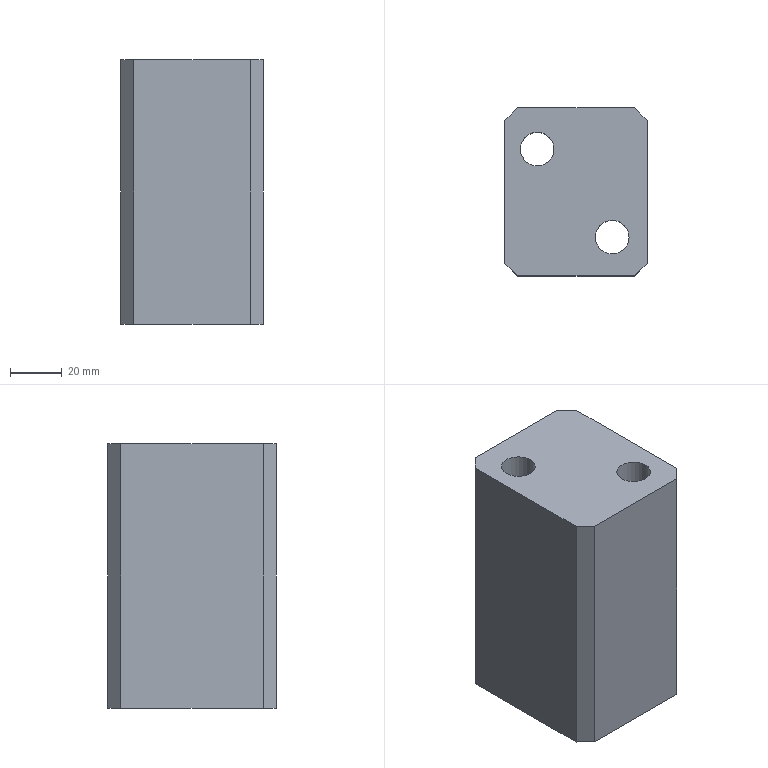Part | STEP file | gslz 2016.10.28-10_id2074_x_t | 1 solid | 22 faces | box 55 x 65 x 102 mm | volume 303943 mm3 | plane 12 | cylinder 6 | cone 4 | commonest cylinder face diameters 10.3 x2 13 x2 20 x2
STEP:
#1=CARTESIAN_POINT('',(0.,0.,0.));
#2=DIRECTION('',(0.,0.,1.));
#3=DIRECTION('',(1.,0.,0.));
#4=AXIS2_PLACEMENT_3D('',#1,#2,#3);
#5=CARTESIAN_POINT('',(512.5,-304.,3.));
#6=VERTEX_POINT('',#5);
#7=CARTESIAN_POINT('',(506.5,-304.,3.));
#8=DIRECTION('',(0.,0.,-1.));
#9=DIRECTION('',(1.,0.,0.));
#10=AXIS2_PLACEMENT_3D('',#7,#8,#9);
#11=CIRCLE('',#10,6.);
#12=CARTESIAN_POINT('',(501.5,-310.,3.));
#13=DIRECTION('',(0.,0.,1.));
#14=DIRECTION('',(0.,-1.,0.));
#15=AXIS2_PLACEMENT_3D('',#12,#13,#14);
#16=PLANE('',#15);
#17=CARTESIAN_POINT('',(-6.,11.));
#18=CARTESIAN_POINT('',(4.392,11.));
#19=CARTESIAN_POINT('',(-0.8038,2.));
#20=CARTESIAN_POINT('',(-6.,-7.));
#21=CARTESIAN_POINT('',(-11.196,2.));
#22=CARTESIAN_POINT('',(-16.392,11.));
#23=CARTESIAN_POINT('',(-6.,11.));
#24=(BOUNDED_CURVE()B_SPLINE_CURVE(2,(#17,#18,#19,#20,#21,#22,#23),.UNSPECIFIED.,.T.,.F.)B_SPLINE_CURVE_WITH_KNOTS((1,2,2,2,2,1),(-2.094,0.,2.094,4.189,6.283,8.378),.UNSPECIFIED.)CURVE()GEOMETRIC_REPRESENTATION_ITEM()RATIONAL_B_SPLINE_CURVE((1.,0.5,1.,0.5,1.,0.5,1.))REPRESENTATION_ITEM(''));
#25=(GEOMETRIC_REPRESENTATION_CONTEXT(2)PARAMETRIC_REPRESENTATION_CONTEXT()REPRESENTATION_CONTEXT('',''));
#26=DEFINITIONAL_REPRESENTATION('',(#24),#25);
#27=PCURVE('',#16,#26);
#28=CARTESIAN_POINT('',(506.5,-304.,3.));
#29=DIRECTION('',(0.,0.,-1.));
#30=DIRECTION('',(1.,0.,0.));
#31=AXIS2_PLACEMENT_3D('',#28,#29,#30);
#32=CONICAL_SURFACE('',#31,6.,0.7854);
#33=CARTESIAN_POINT('',(0.,0.));
#34=DIRECTION('',(1.,0.));
#35=VECTOR('',#34,1.);
#36=LINE('',#33,#35);
#37=(GEOMETRIC_REPRESENTATION_CONTEXT(2)PARAMETRIC_REPRESENTATION_CONTEXT()REPRESENTATION_CONTEXT('',''));
#38=DEFINITIONAL_REPRESENTATION('',(#36),#37);
#39=PCURVE('',#32,#38);
#40=SURFACE_CURVE('',#11,(#27,#39),.PCURVE_S1.);
#41=EDGE_CURVE('',#6,#6,#40,.T.);
#42=ORIENTED_EDGE('',*,*,#41,.F.);
#43=EDGE_LOOP('',(#42));
#44=FACE_BOUND('',#43,.T.);
#45=CARTESIAN_POINT('',(541.5,-269.,3.));
#46=VERTEX_POINT('',#45);
#47=CARTESIAN_POINT('',(535.5,-269.,3.));
#48=DIRECTION('',(0.,0.,-1.));
#49=DIRECTION('',(1.,0.,0.));
#50=AXIS2_PLACEMENT_3D('',#47,#48,#49);
#51=CIRCLE('',#50,6.);
#52=CARTESIAN_POINT('',(-41.,40.));
#53=CARTESIAN_POINT('',(-30.608,40.));
#54=CARTESIAN_POINT('',(-35.804,31.));
#55=CARTESIAN_POINT('',(-41.,22.));
#56=CARTESIAN_POINT('',(-46.196,31.));
#57=CARTESIAN_POINT('',(-51.392,40.));
#58=CARTESIAN_POINT('',(-41.,40.));
#59=(BOUNDED_CURVE()B_SPLINE_CURVE(2,(#52,#53,#54,#55,#56,#57,#58),.UNSPECIFIED.,.T.,.F.)B_SPLINE_CURVE_WITH_KNOTS((1,2,2,2,2,1),(-2.094,0.,2.094,4.189,6.283,8.378),.UNSPECIFIED.)CURVE()GEOMETRIC_REPRESENTATION_ITEM()RATIONAL_B_SPLINE_CURVE((1.,0.5,1.,0.5,1.,0.5,1.))REPRESENTATION_ITEM(''));
#60=(GEOMETRIC_REPRESENTATION_CONTEXT(2)PARAMETRIC_REPRESENTATION_CONTEXT()REPRESENTATION_CONTEXT('',''));
#61=DEFINITIONAL_REPRESENTATION('',(#59),#60);
#62=PCURVE('',#16,#61);
#63=CARTESIAN_POINT('',(535.5,-269.,3.));
#64=DIRECTION('',(0.,0.,-1.));
#65=DIRECTION('',(1.,0.,0.));
#66=AXIS2_PLACEMENT_3D('',#63,#64,#65);
#67=CONICAL_SURFACE('',#66,6.,0.7854);
#68=CARTESIAN_POINT('',(0.,0.));
#69=DIRECTION('',(1.,0.));
#70=VECTOR('',#69,1.);
#71=LINE('',#68,#70);
#72=(GEOMETRIC_REPRESENTATION_CONTEXT(2)PARAMETRIC_REPRESENTATION_CONTEXT()REPRESENTATION_CONTEXT('',''));
#73=DEFINITIONAL_REPRESENTATION('',(#71),#72);
#74=PCURVE('',#67,#73);
#75=SURFACE_CURVE('',#51,(#62,#74),.PCURVE_S1.);
#76=EDGE_CURVE('',#46,#46,#75,.T.);
#77=ORIENTED_EDGE('',*,*,#76,.F.);
#78=EDGE_LOOP('',(#77));
#79=FACE_BOUND('',#78,.T.);
#80=CARTESIAN_POINT('',(535.5,-313.,3.));
#81=VERTEX_POINT('',#80);
#82=CARTESIAN_POINT('',(545.5,-303.,3.));
#83=VERTEX_POINT('',#82);
#84=CARTESIAN_POINT('',(535.5,-303.,3.));
#85=DIRECTION('',(0.,0.,1.));
#86=DIRECTION('',(0.,-1.,0.));
#87=AXIS2_PLACEMENT_3D('',#84,#85,#86);
#88=CIRCLE('',#87,10.);
#89=CARTESIAN_POINT('',(-7.,34.));
#90=DIRECTION('',(1.,0.));
#91=AXIS2_PLACEMENT_2D('',#89,#90);
#92=CIRCLE('',#91,10.);
#93=(GEOMETRIC_REPRESENTATION_CONTEXT(2)PARAMETRIC_REPRESENTATION_CONTEXT()REPRESENTATION_CONTEXT('',''));
#94=DEFINITIONAL_REPRESENTATION('',(#92),#93);
#95=PCURVE('',#16,#94);
#96=CARTESIAN_POINT('',(535.5,-303.,42.));
#97=DIRECTION('',(0.,0.,1.));
#98=DIRECTION('',(1.,0.,0.));
#99=AXIS2_PLACEMENT_3D('',#96,#97,#98);
#100=CYLINDRICAL_SURFACE('',#99,10.);
#101=CARTESIAN_POINT('',(4.712,-39.));
#102=DIRECTION('',(1.,0.));
#103=VECTOR('',#102,1.);
#104=LINE('',#101,#103);
#105=(GEOMETRIC_REPRESENTATION_CONTEXT(2)PARAMETRIC_REPRESENTATION_CONTEXT()REPRESENTATION_CONTEXT('',''));
#106=DEFINITIONAL_REPRESENTATION('',(#104),#105);
#107=PCURVE('',#100,#106);
#108=SURFACE_CURVE('',#88,(#95,#107),.PCURVE_S1.);
#109=EDGE_CURVE('',#81,#83,#108,.T.);
#110=ORIENTED_EDGE('',*,*,#109,.T.);
#111=CARTESIAN_POINT('',(535.5,-303.,3.));
#112=DIRECTION('',(0.,0.,1.));
#113=DIRECTION('',(0.,-1.,0.));
#114=AXIS2_PLACEMENT_3D('',#111,#112,#113);
#115=CIRCLE('',#114,10.);
#116=CARTESIAN_POINT('',(-7.,34.));
#117=DIRECTION('',(1.,0.));
#118=AXIS2_PLACEMENT_2D('',#116,#117);
#119=CIRCLE('',#118,10.);
#120=(GEOMETRIC_REPRESENTATION_CONTEXT(2)PARAMETRIC_REPRESENTATION_CONTEXT()REPRESENTATION_CONTEXT('',''));
#121=DEFINITIONAL_REPRESENTATION('',(#119),#120);
#122=PCURVE('',#16,#121);
#123=CARTESIAN_POINT('',(-1.571,-39.));
#124=DIRECTION('',(1.,0.));
#125=VECTOR('',#124,1.);
#126=LINE('',#123,#125);
#127=(GEOMETRIC_REPRESENTATION_CONTEXT(2)PARAMETRIC_REPRESENTATION_CONTEXT()REPRESENTATION_CONTEXT('',''));
#128=DEFINITIONAL_REPRESENTATION('',(#126),#127);
#129=PCURVE('',#100,#128);
#130=SURFACE_CURVE('',#115,(#122,#129),.PCURVE_S1.);
#131=EDGE_CURVE('',#83,#81,#130,.T.);
#132=ORIENTED_EDGE('',*,*,#131,.T.);
#133=EDGE_LOOP('',(#110,#132));
#134=FACE_BOUND('',#133,.T.);
#135=CARTESIAN_POINT('',(494.,-257.929,3.));
#136=VERTEX_POINT('',#135);
#137=CARTESIAN_POINT('',(494.,-313.071,3.));
#138=VERTEX_POINT('',#137);
#139=CARTESIAN_POINT('',(494.,622.983,3.));
#140=DIRECTION('',(0.,-1.,0.));
#141=VECTOR('',#140,1.);
#142=LINE('',#139,#141);
#143=CARTESIAN_POINT('',(-932.983,-7.5));
#144=DIRECTION('',(1.,0.));
#145=VECTOR('',#144,1.);
#146=LINE('',#143,#145);
#147=(GEOMETRIC_REPRESENTATION_CONTEXT(2)PARAMETRIC_REPRESENTATION_CONTEXT()REPRESENTATION_CONTEXT('',''));
#148=DEFINITIONAL_REPRESENTATION('',(#146),#147);
#149=PCURVE('',#16,#148);
#150=CARTESIAN_POINT('',(494.,622.983,98.));
#151=DIRECTION('',(-1.,0.,0.));
#152=DIRECTION('',(0.,0.,1.));
#153=AXIS2_PLACEMENT_3D('',#150,#151,#152);
#154=PLANE('',#153);
#155=CARTESIAN_POINT('',(-95.,0.));
#156=DIRECTION('',(0.,-1.));
#157=VECTOR('',#156,1.);
#158=LINE('',#155,#157);
#159=(GEOMETRIC_REPRESENTATION_CONTEXT(2)PARAMETRIC_REPRESENTATION_CONTEXT()REPRESENTATION_CONTEXT('',''));
#160=DEFINITIONAL_REPRESENTATION('',(#158),#159);
#161=PCURVE('',#154,#160);
#162=SURFACE_CURVE('',#142,(#149,#161),.PCURVE_S1.);
#163=EDGE_CURVE('',#136,#138,#162,.T.);
#164=ORIENTED_EDGE('',*,*,#163,.F.);
#165=CARTESIAN_POINT('',(498.929,-253.,3.));
#166=VERTEX_POINT('',#165);
#167=CARTESIAN_POINT('',(497.464,-254.464,3.));
#168=DIRECTION('',(-0.7071,-0.7071,0.));
#169=VECTOR('',#168,1.);
#170=LINE('',#167,#169);
#171=CARTESIAN_POINT('',(-55.536,-4.036));
#172=DIRECTION('',(0.7071,-0.7071));
#173=VECTOR('',#172,1.);
#174=LINE('',#171,#173);
#175=(GEOMETRIC_REPRESENTATION_CONTEXT(2)PARAMETRIC_REPRESENTATION_CONTEXT()REPRESENTATION_CONTEXT('',''));
#176=DEFINITIONAL_REPRESENTATION('',(#174),#175);
#177=PCURVE('',#16,#176);
#178=CARTESIAN_POINT('',(497.464,-254.464,98.));
#179=DIRECTION('',(0.7071,-0.7071,0.));
#180=DIRECTION('',(0.,0.,1.));
#181=AXIS2_PLACEMENT_3D('',#178,#179,#180);
#182=PLANE('',#181);
#183=CARTESIAN_POINT('',(-95.,0.));
#184=DIRECTION('',(0.,1.));
#185=VECTOR('',#184,1.);
#186=LINE('',#183,#185);
#187=(GEOMETRIC_REPRESENTATION_CONTEXT(2)PARAMETRIC_REPRESENTATION_CONTEXT()REPRESENTATION_CONTEXT('',''));
#188=DEFINITIONAL_REPRESENTATION('',(#186),#187);
#189=PCURVE('',#182,#188);
#190=SURFACE_CURVE('',#170,(#177,#189),.PCURVE_S1.);
#191=EDGE_CURVE('',#166,#136,#190,.T.);
#192=ORIENTED_EDGE('',*,*,#191,.F.);
#193=CARTESIAN_POINT('',(544.071,-253.,3.));
#194=VERTEX_POINT('',#193);
#195=CARTESIAN_POINT('',(-137.884,-253.,3.));
#196=DIRECTION('',(-1.,0.,0.));
#197=VECTOR('',#196,1.);
#198=LINE('',#195,#197);
#199=CARTESIAN_POINT('',(-57.,-639.384));
#200=DIRECTION('',(0.,-1.));
#201=VECTOR('',#200,1.);
#202=LINE('',#199,#201);
#203=(GEOMETRIC_REPRESENTATION_CONTEXT(2)PARAMETRIC_REPRESENTATION_CONTEXT()REPRESENTATION_CONTEXT('',''));
#204=DEFINITIONAL_REPRESENTATION('',(#202),#203);
#205=PCURVE('',#16,#204);
#206=CARTESIAN_POINT('',(-137.884,-253.,98.));
#207=DIRECTION('',(0.,1.,0.));
#208=DIRECTION('',(1.,0.,0.));
#209=AXIS2_PLACEMENT_3D('',#206,#207,#208);
#210=PLANE('',#209);
#211=CARTESIAN_POINT('',(0.,95.));
#212=DIRECTION('',(-1.,0.));
#213=VECTOR('',#212,1.);
#214=LINE('',#211,#213);
#215=(GEOMETRIC_REPRESENTATION_CONTEXT(2)PARAMETRIC_REPRESENTATION_CONTEXT()REPRESENTATION_CONTEXT('',''));
#216=DEFINITIONAL_REPRESENTATION('',(#214),#215);
#217=PCURVE('',#210,#216);
#218=SURFACE_CURVE('',#198,(#205,#217),.PCURVE_S1.);
#219=EDGE_CURVE('',#194,#166,#218,.T.);
#220=ORIENTED_EDGE('',*,*,#219,.F.);
#221=CARTESIAN_POINT('',(549.,-257.929,3.));
#222=VERTEX_POINT('',#221);
#223=CARTESIAN_POINT('',(547.536,-256.464,3.));
#224=DIRECTION('',(-0.7071,0.7071,0.));
#225=VECTOR('',#224,1.);
#226=LINE('',#223,#225);
#227=CARTESIAN_POINT('',(-53.536,46.036));
#228=DIRECTION('',(-0.7071,-0.7071));
#229=VECTOR('',#228,1.);
#230=LINE('',#227,#229);
#231=(GEOMETRIC_REPRESENTATION_CONTEXT(2)PARAMETRIC_REPRESENTATION_CONTEXT()REPRESENTATION_CONTEXT('',''));
#232=DEFINITIONAL_REPRESENTATION('',(#230),#231);
#233=PCURVE('',#16,#232);
#234=CARTESIAN_POINT('',(547.536,-256.464,98.));
#235=DIRECTION('',(-0.7071,-0.7071,0.));
#236=DIRECTION('',(0.,0.,1.));
#237=AXIS2_PLACEMENT_3D('',#234,#235,#236);
#238=PLANE('',#237);
#239=CARTESIAN_POINT('',(-95.,0.));
#240=DIRECTION('',(0.,1.));
#241=VECTOR('',#240,1.);
#242=LINE('',#239,#241);
#243=(GEOMETRIC_REPRESENTATION_CONTEXT(2)PARAMETRIC_REPRESENTATION_CONTEXT()REPRESENTATION_CONTEXT('',''));
#244=DEFINITIONAL_REPRESENTATION('',(#242),#243);
#245=PCURVE('',#238,#244);
#246=SURFACE_CURVE('',#226,(#233,#245),.PCURVE_S1.);
#247=EDGE_CURVE('',#222,#194,#246,.T.);
#248=ORIENTED_EDGE('',*,*,#247,.F.);
#249=CARTESIAN_POINT('',(549.,-313.071,3.));
#250=VERTEX_POINT('',#249);
#251=CARTESIAN_POINT('',(549.,622.983,3.));
#252=DIRECTION('',(0.,1.,0.));
#253=VECTOR('',#252,1.);
#254=LINE('',#251,#253);
#255=CARTESIAN_POINT('',(-932.983,47.5));
#256=DIRECTION('',(-1.,0.));
#257=VECTOR('',#256,1.);
#258=LINE('',#255,#257);
#259=(GEOMETRIC_REPRESENTATION_CONTEXT(2)PARAMETRIC_REPRESENTATION_CONTEXT()REPRESENTATION_CONTEXT('',''));
#260=DEFINITIONAL_REPRESENTATION('',(#258),#259);
#261=PCURVE('',#16,#260);
#262=CARTESIAN_POINT('',(549.,622.983,98.));
#263=DIRECTION('',(1.,0.,0.));
#264=DIRECTION('',(0.,0.,-1.));
#265=AXIS2_PLACEMENT_3D('',#262,#263,#264);
#266=PLANE('',#265);
#267=CARTESIAN_POINT('',(95.,0.));
#268=DIRECTION('',(0.,1.));
#269=VECTOR('',#268,1.);
#270=LINE('',#267,#269);
#271=(GEOMETRIC_REPRESENTATION_CONTEXT(2)PARAMETRIC_REPRESENTATION_CONTEXT()REPRESENTATION_CONTEXT('',''));
#272=DEFINITIONAL_REPRESENTATION('',(#270),#271);
#273=PCURVE('',#266,#272);
#274=SURFACE_CURVE('',#254,(#261,#273),.PCURVE_S1.);
#275=EDGE_CURVE('',#250,#222,#274,.T.);
#276=ORIENTED_EDGE('',*,*,#275,.F.);
#277=CARTESIAN_POINT('',(544.071,-318.,3.));
#278=VERTEX_POINT('',#277);
#279=CARTESIAN_POINT('',(547.536,-314.536,3.));
#280=DIRECTION('',(0.7071,0.7071,0.));
#281=VECTOR('',#280,1.);
#282=LINE('',#279,#281);
#283=CARTESIAN_POINT('',(4.536,46.036));
#284=DIRECTION('',(-0.7071,0.7071));
#285=VECTOR('',#284,1.);
#286=LINE('',#283,#285);
#287=(GEOMETRIC_REPRESENTATION_CONTEXT(2)PARAMETRIC_REPRESENTATION_CONTEXT()REPRESENTATION_CONTEXT('',''));
#288=DEFINITIONAL_REPRESENTATION('',(#286),#287);
#289=PCURVE('',#16,#288);
#290=CARTESIAN_POINT('',(547.536,-314.536,98.));
#291=DIRECTION('',(-0.7071,0.7071,0.));
#292=DIRECTION('',(0.,0.,-1.));
#293=AXIS2_PLACEMENT_3D('',#290,#291,#292);
#294=PLANE('',#293);
#295=CARTESIAN_POINT('',(95.,0.));
#296=DIRECTION('',(0.,-1.));
#297=VECTOR('',#296,1.);
#298=LINE('',#295,#297);
#299=(GEOMETRIC_REPRESENTATION_CONTEXT(2)PARAMETRIC_REPRESENTATION_CONTEXT()REPRESENTATION_CONTEXT('',''));
#300=DEFINITIONAL_REPRESENTATION('',(#298),#299);
#301=PCURVE('',#294,#300);
#302=SURFACE_CURVE('',#282,(#289,#301),.PCURVE_S1.);
#303=EDGE_CURVE('',#278,#250,#302,.T.);
#304=ORIENTED_EDGE('',*,*,#303,.F.);
#305=CARTESIAN_POINT('',(498.929,-318.,3.));
#306=VERTEX_POINT('',#305);
#307=CARTESIAN_POINT('',(-137.035,-318.,3.));
#308=DIRECTION('',(1.,0.,0.));
#309=VECTOR('',#308,1.);
#310=LINE('',#307,#309);
#311=CARTESIAN_POINT('',(8.,-638.535));
#312=DIRECTION('',(0.,1.));
#313=VECTOR('',#312,1.);
#314=LINE('',#311,#313);
#315=(GEOMETRIC_REPRESENTATION_CONTEXT(2)PARAMETRIC_REPRESENTATION_CONTEXT()REPRESENTATION_CONTEXT('',''));
#316=DEFINITIONAL_REPRESENTATION('',(#314),#315);
#317=PCURVE('',#16,#316);
#318=CARTESIAN_POINT('',(-137.035,-318.,98.));
#319=DIRECTION('',(0.,-1.,0.));
#320=DIRECTION('',(-1.,0.,0.));
#321=AXIS2_PLACEMENT_3D('',#318,#319,#320);
#322=PLANE('',#321);
#323=CARTESIAN_POINT('',(0.,95.));
#324=DIRECTION('',(-1.,0.));
#325=VECTOR('',#324,1.);
#326=LINE('',#323,#325);
#327=(GEOMETRIC_REPRESENTATION_CONTEXT(2)PARAMETRIC_REPRESENTATION_CONTEXT()REPRESENTATION_CONTEXT('',''));
#328=DEFINITIONAL_REPRESENTATION('',(#326),#327);
#329=PCURVE('',#322,#328);
#330=SURFACE_CURVE('',#310,(#317,#329),.PCURVE_S1.);
#331=EDGE_CURVE('',#306,#278,#330,.T.);
#332=ORIENTED_EDGE('',*,*,#331,.F.);
#333=CARTESIAN_POINT('',(497.464,-316.536,3.));
#334=DIRECTION('',(0.7071,-0.7071,0.));
#335=VECTOR('',#334,1.);
#336=LINE('',#333,#335);
#337=CARTESIAN_POINT('',(6.536,-4.036));
#338=DIRECTION('',(0.7071,0.7071));
#339=VECTOR('',#338,1.);
#340=LINE('',#337,#339);
#341=(GEOMETRIC_REPRESENTATION_CONTEXT(2)PARAMETRIC_REPRESENTATION_CONTEXT()REPRESENTATION_CONTEXT('',''));
#342=DEFINITIONAL_REPRESENTATION('',(#340),#341);
#343=PCURVE('',#16,#342);
#344=CARTESIAN_POINT('',(497.464,-316.536,98.));
#345=DIRECTION('',(0.7071,0.7071,0.));
#346=DIRECTION('',(0.,0.,-1.));
#347=AXIS2_PLACEMENT_3D('',#344,#345,#346);
#348=PLANE('',#347);
#349=CARTESIAN_POINT('',(95.,0.));
#350=DIRECTION('',(0.,-1.));
#351=VECTOR('',#350,1.);
#352=LINE('',#349,#351);
#353=(GEOMETRIC_REPRESENTATION_CONTEXT(2)PARAMETRIC_REPRESENTATION_CONTEXT()REPRESENTATION_CONTEXT('',''));
#354=DEFINITIONAL_REPRESENTATION('',(#352),#353);
#355=PCURVE('',#348,#354);
#356=SURFACE_CURVE('',#336,(#343,#355),.PCURVE_S1.);
#357=EDGE_CURVE('',#138,#306,#356,.T.);
#358=ORIENTED_EDGE('',*,*,#357,.F.);
#359=EDGE_LOOP('',(#164,#192,#220,#248,#276,#304,#332,#358));
#360=FACE_BOUND('',#359,.T.);
#361=CARTESIAN_POINT('',(506.5,-279.,3.));
#362=VERTEX_POINT('',#361);
#363=CARTESIAN_POINT('',(516.5,-269.,3.));
#364=VERTEX_POINT('',#363);
#365=CARTESIAN_POINT('',(506.5,-269.,3.));
#366=DIRECTION('',(0.,0.,1.));
#367=DIRECTION('',(0.,-1.,0.));
#368=AXIS2_PLACEMENT_3D('',#365,#366,#367);
#369=CIRCLE('',#368,10.);
#370=CARTESIAN_POINT('',(-41.,5.));
#371=DIRECTION('',(1.,0.));
#372=AXIS2_PLACEMENT_2D('',#370,#371);
#373=CIRCLE('',#372,10.);
#374=(GEOMETRIC_REPRESENTATION_CONTEXT(2)PARAMETRIC_REPRESENTATION_CONTEXT()REPRESENTATION_CONTEXT('',''));
#375=DEFINITIONAL_REPRESENTATION('',(#373),#374);
#376=PCURVE('',#16,#375);
#377=CARTESIAN_POINT('',(506.5,-269.,42.));
#378=DIRECTION('',(0.,0.,1.));
#379=DIRECTION('',(1.,0.,0.));
#380=AXIS2_PLACEMENT_3D('',#377,#378,#379);
#381=CYLINDRICAL_SURFACE('',#380,10.);
#382=CARTESIAN_POINT('',(4.712,-39.));
#383=DIRECTION('',(1.,0.));
#384=VECTOR('',#383,1.);
#385=LINE('',#382,#384);
#386=(GEOMETRIC_REPRESENTATION_CONTEXT(2)PARAMETRIC_REPRESENTATION_CONTEXT()REPRESENTATION_CONTEXT('',''));
#387=DEFINITIONAL_REPRESENTATION('',(#385),#386);
#388=PCURVE('',#381,#387);
#389=SURFACE_CURVE('',#369,(#376,#388),.PCURVE_S1.);
#390=EDGE_CURVE('',#362,#364,#389,.T.);
#391=ORIENTED_EDGE('',*,*,#390,.T.);
#392=CARTESIAN_POINT('',(506.5,-269.,3.));
#393=DIRECTION('',(0.,0.,1.));
#394=DIRECTION('',(0.,-1.,0.));
#395=AXIS2_PLACEMENT_3D('',#392,#393,#394);
#396=CIRCLE('',#395,10.);
#397=CARTESIAN_POINT('',(-41.,5.));
#398=DIRECTION('',(1.,0.));
#399=AXIS2_PLACEMENT_2D('',#397,#398);
#400=CIRCLE('',#399,10.);
#401=(GEOMETRIC_REPRESENTATION_CONTEXT(2)PARAMETRIC_REPRESENTATION_CONTEXT()REPRESENTATION_CONTEXT('',''));
#402=DEFINITIONAL_REPRESENTATION('',(#400),#401);
#403=PCURVE('',#16,#402);
#404=CARTESIAN_POINT('',(-1.571,-39.));
#405=DIRECTION('',(1.,0.));
#406=VECTOR('',#405,1.);
#407=LINE('',#404,#406);
#408=(GEOMETRIC_REPRESENTATION_CONTEXT(2)PARAMETRIC_REPRESENTATION_CONTEXT()REPRESENTATION_CONTEXT('',''));
#409=DEFINITIONAL_REPRESENTATION('',(#407),#408);
#410=PCURVE('',#381,#409);
#411=SURFACE_CURVE('',#396,(#403,#410),.PCURVE_S1.);
#412=EDGE_CURVE('',#364,#362,#411,.T.);
#413=ORIENTED_EDGE('',*,*,#412,.T.);
#414=EDGE_LOOP('',(#391,#413));
#415=FACE_BOUND('',#414,.T.);
#416=ADVANCED_FACE('',(#44,#79,#134,#360,#415),#16,.F.);
#417=CARTESIAN_POINT('',(542.,-303.,70.));
#418=VERTEX_POINT('',#417);
#419=CARTESIAN_POINT('',(535.5,-303.,70.));
#420=DIRECTION('',(0.,0.,1.));
#421=DIRECTION('',(1.,0.,0.));
#422=AXIS2_PLACEMENT_3D('',#419,#420,#421);
#423=CIRCLE('',#422,6.5);
#424=CARTESIAN_POINT('',(535.5,-303.,70.));
#425=DIRECTION('',(0.,0.,1.));
#426=DIRECTION('',(1.,0.,0.));
#427=AXIS2_PLACEMENT_3D('',#424,#425,#426);
#428=PLANE('',#427);
#429=CARTESIAN_POINT('',(0.,0.));
#430=DIRECTION('',(1.,0.));
#431=AXIS2_PLACEMENT_2D('',#429,#430);
#432=CIRCLE('',#431,6.5);
#433=(GEOMETRIC_REPRESENTATION_CONTEXT(2)PARAMETRIC_REPRESENTATION_CONTEXT()REPRESENTATION_CONTEXT('',''));
#434=DEFINITIONAL_REPRESENTATION('',(#432),#433);
#435=PCURVE('',#428,#434);
#436=CARTESIAN_POINT('',(535.5,-303.,87.));
#437=DIRECTION('',(0.,0.,1.));
#438=DIRECTION('',(1.,0.,0.));
#439=AXIS2_PLACEMENT_3D('',#436,#437,#438);
#440=CYLINDRICAL_SURFACE('',#439,6.5);
#441=CARTESIAN_POINT('',(0.,-17.));
#442=DIRECTION('',(1.,0.));
#443=VECTOR('',#442,1.);
#444=LINE('',#441,#443);
#445=(GEOMETRIC_REPRESENTATION_CONTEXT(2)PARAMETRIC_REPRESENTATION_CONTEXT()REPRESENTATION_CONTEXT('',''));
#446=DEFINITIONAL_REPRESENTATION('',(#444),#445);
#447=PCURVE('',#440,#446);
#448=SURFACE_CURVE('',#423,(#435,#447),.PCURVE_S1.);
#449=EDGE_CURVE('',#418,#418,#448,.T.);
#450=ORIENTED_EDGE('',*,*,#449,.T.);
#451=EDGE_LOOP('',(#450));
#452=FACE_BOUND('',#451,.T.);
#453=CARTESIAN_POINT('',(545.5,-303.,70.));
#454=VERTEX_POINT('',#453);
#455=CARTESIAN_POINT('',(535.5,-303.,70.));
#456=DIRECTION('',(0.,0.,1.));
#457=DIRECTION('',(1.,0.,0.));
#458=AXIS2_PLACEMENT_3D('',#455,#456,#457);
#459=CIRCLE('',#458,10.);
#460=CARTESIAN_POINT('',(0.,0.));
#461=DIRECTION('',(1.,0.));
#462=AXIS2_PLACEMENT_2D('',#460,#461);
#463=CIRCLE('',#462,10.);
#464=(GEOMETRIC_REPRESENTATION_CONTEXT(2)PARAMETRIC_REPRESENTATION_CONTEXT()REPRESENTATION_CONTEXT('',''));
#465=DEFINITIONAL_REPRESENTATION('',(#463),#464);
#466=PCURVE('',#428,#465);
#467=CARTESIAN_POINT('',(0.,28.));
#468=DIRECTION('',(1.,0.));
#469=VECTOR('',#468,1.);
#470=LINE('',#467,#469);
#471=(GEOMETRIC_REPRESENTATION_CONTEXT(2)PARAMETRIC_REPRESENTATION_CONTEXT()REPRESENTATION_CONTEXT('',''));
#472=DEFINITIONAL_REPRESENTATION('',(#470),#471);
#473=PCURVE('',#100,#472);
#474=SURFACE_CURVE('',#459,(#466,#473),.PCURVE_S1.);
#475=EDGE_CURVE('',#454,#454,#474,.T.);
#476=ORIENTED_EDGE('',*,*,#475,.F.);
#477=EDGE_LOOP('',(#476));
#478=FACE_BOUND('',#477,.T.);
#479=ADVANCED_FACE('',(#452,#478),#428,.F.);
#480=CARTESIAN_POINT('',(513.,-269.,70.));
#481=VERTEX_POINT('',#480);
#482=CARTESIAN_POINT('',(506.5,-269.,70.));
#483=DIRECTION('',(0.,0.,1.));
#484=DIRECTION('',(1.,0.,0.));
#485=AXIS2_PLACEMENT_3D('',#482,#483,#484);
#486=CIRCLE('',#485,6.5);
#487=CARTESIAN_POINT('',(506.5,-269.,70.));
#488=DIRECTION('',(0.,0.,1.));
#489=DIRECTION('',(1.,0.,0.));
#490=AXIS2_PLACEMENT_3D('',#487,#488,#489);
#491=PLANE('',#490);
#492=CARTESIAN_POINT('',(0.,0.));
#493=DIRECTION('',(1.,0.));
#494=AXIS2_PLACEMENT_2D('',#492,#493);
#495=CIRCLE('',#494,6.5);
#496=(GEOMETRIC_REPRESENTATION_CONTEXT(2)PARAMETRIC_REPRESENTATION_CONTEXT()REPRESENTATION_CONTEXT('',''));
#497=DEFINITIONAL_REPRESENTATION('',(#495),#496);
#498=PCURVE('',#491,#497);
#499=CARTESIAN_POINT('',(506.5,-269.,87.));
#500=DIRECTION('',(0.,0.,1.));
#501=DIRECTION('',(1.,0.,0.));
#502=AXIS2_PLACEMENT_3D('',#499,#500,#501);
#503=CYLINDRICAL_SURFACE('',#502,6.5);
#504=CARTESIAN_POINT('',(0.,-17.));
#505=DIRECTION('',(1.,0.));
#506=VECTOR('',#505,1.);
#507=LINE('',#504,#506);
#508=(GEOMETRIC_REPRESENTATION_CONTEXT(2)PARAMETRIC_REPRESENTATION_CONTEXT()REPRESENTATION_CONTEXT('',''));
#509=DEFINITIONAL_REPRESENTATION('',(#507),#508);
#510=PCURVE('',#503,#509);
#511=SURFACE_CURVE('',#486,(#498,#510),.PCURVE_S1.);
#512=EDGE_CURVE('',#481,#481,#511,.T.);
#513=ORIENTED_EDGE('',*,*,#512,.T.);
#514=EDGE_LOOP('',(#513));
#515=FACE_BOUND('',#514,.T.);
#516=CARTESIAN_POINT('',(516.5,-269.,70.));
#517=VERTEX_POINT('',#516);
#518=CARTESIAN_POINT('',(506.5,-269.,70.));
#519=DIRECTION('',(0.,0.,1.));
#520=DIRECTION('',(1.,0.,0.));
#521=AXIS2_PLACEMENT_3D('',#518,#519,#520);
#522=CIRCLE('',#521,10.);
#523=CARTESIAN_POINT('',(0.,0.));
#524=DIRECTION('',(1.,0.));
#525=AXIS2_PLACEMENT_2D('',#523,#524);
#526=CIRCLE('',#525,10.);
#527=(GEOMETRIC_REPRESENTATION_CONTEXT(2)PARAMETRIC_REPRESENTATION_CONTEXT()REPRESENTATION_CONTEXT('',''));
#528=DEFINITIONAL_REPRESENTATION('',(#526),#527);
#529=PCURVE('',#491,#528);
#530=CARTESIAN_POINT('',(0.,28.));
#531=DIRECTION('',(1.,0.));
#532=VECTOR('',#531,1.);
#533=LINE('',#530,#532);
#534=(GEOMETRIC_REPRESENTATION_CONTEXT(2)PARAMETRIC_REPRESENTATION_CONTEXT()REPRESENTATION_CONTEXT('',''));
#535=DEFINITIONAL_REPRESENTATION('',(#533),#534);
#536=PCURVE('',#381,#535);
#537=SURFACE_CURVE('',#522,(#529,#536),.PCURVE_S1.);
#538=EDGE_CURVE('',#517,#517,#537,.T.);
#539=ORIENTED_EDGE('',*,*,#538,.F.);
#540=EDGE_LOOP('',(#539));
#541=FACE_BOUND('',#540,.T.);
#542=ADVANCED_FACE('',(#515,#541),#491,.F.);
#543=ORIENTED_EDGE('',*,*,#109,.T.);
#544=CARTESIAN_POINT('',(545.5,-303.,3.));
#545=CARTESIAN_POINT('',(545.5,-303.,70.));
#546=B_SPLINE_CURVE_WITH_KNOTS('',1,(#544,#545),.UNSPECIFIED.,.F.,.F.,(2,2),(-39.,28.),.PIECEWISE_BEZIER_KNOTS.);
#547=CARTESIAN_POINT('',(6.283,0.));
#548=DIRECTION('',(0.,1.));
#549=VECTOR('',#548,1.);
#550=LINE('',#547,#549);
#551=(GEOMETRIC_REPRESENTATION_CONTEXT(2)PARAMETRIC_REPRESENTATION_CONTEXT()REPRESENTATION_CONTEXT('',''));
#552=DEFINITIONAL_REPRESENTATION('',(#550),#551);
#553=PCURVE('',#100,#552);
#554=CARTESIAN_POINT('',(0.,0.));
#555=DIRECTION('',(0.,1.));
#556=VECTOR('',#555,1.);
#557=LINE('',#554,#556);
#558=(GEOMETRIC_REPRESENTATION_CONTEXT(2)PARAMETRIC_REPRESENTATION_CONTEXT()REPRESENTATION_CONTEXT('',''));
#559=DEFINITIONAL_REPRESENTATION('',(#557),#558);
#560=PCURVE('',#100,#559);
#561=SEAM_CURVE('',#546,(#553,#560),.PCURVE_S1.);
#562=EDGE_CURVE('',#83,#454,#561,.T.);
#563=ORIENTED_EDGE('',*,*,#562,.T.);
#564=ORIENTED_EDGE('',*,*,#475,.F.);
#565=ORIENTED_EDGE('',*,*,#562,.F.);
#566=ORIENTED_EDGE('',*,*,#131,.T.);
#567=EDGE_LOOP('',(#543,#563,#564,#565,#566));
#568=FACE_BOUND('',#567,.F.);
#569=ADVANCED_FACE('',(#568),#100,.F.);
#570=ORIENTED_EDGE('',*,*,#331,.T.);
#571=CARTESIAN_POINT('',(544.071,-318.,105.));
#572=VERTEX_POINT('',#571);
#573=CARTESIAN_POINT('',(544.071,-318.,98.));
#574=DIRECTION('',(0.,0.,-1.));
#575=VECTOR('',#574,1.);
#576=LINE('',#573,#575);
#577=CARTESIAN_POINT('',(-681.106,0.));
#578=DIRECTION('',(0.,1.));
#579=VECTOR('',#578,1.);
#580=LINE('',#577,#579);
#581=(GEOMETRIC_REPRESENTATION_CONTEXT(2)PARAMETRIC_REPRESENTATION_CONTEXT()REPRESENTATION_CONTEXT('',''));
#582=DEFINITIONAL_REPRESENTATION('',(#580),#581);
#583=PCURVE('',#322,#582);
#584=CARTESIAN_POINT('',(0.,4.899));
#585=DIRECTION('',(1.,0.));
#586=VECTOR('',#585,1.);
#587=LINE('',#584,#586);
#588=(GEOMETRIC_REPRESENTATION_CONTEXT(2)PARAMETRIC_REPRESENTATION_CONTEXT()REPRESENTATION_CONTEXT('',''));
#589=DEFINITIONAL_REPRESENTATION('',(#587),#588);
#590=PCURVE('',#294,#589);
#591=SURFACE_CURVE('',#576,(#583,#590),.PCURVE_S1.);
#592=EDGE_CURVE('',#572,#278,#591,.T.);
#593=ORIENTED_EDGE('',*,*,#592,.F.);
#594=CARTESIAN_POINT('',(498.929,-318.,105.));
#595=VERTEX_POINT('',#594);
#596=CARTESIAN_POINT('',(586.5,-318.,105.));
#597=DIRECTION('',(1.,0.,0.));
#598=VECTOR('',#597,1.);
#599=LINE('',#596,#598);
#600=CARTESIAN_POINT('',(-723.535,-7.));
#601=DIRECTION('',(-1.,0.));
#602=VECTOR('',#601,1.);
#603=LINE('',#600,#602);
#604=(GEOMETRIC_REPRESENTATION_CONTEXT(2)PARAMETRIC_REPRESENTATION_CONTEXT()REPRESENTATION_CONTEXT('',''));
#605=DEFINITIONAL_REPRESENTATION('',(#603),#604);
#606=PCURVE('',#322,#605);
#607=CARTESIAN_POINT('',(586.5,97.,105.));
#608=DIRECTION('',(0.,0.,1.));
#609=DIRECTION('',(-1.,0.,0.));
#610=AXIS2_PLACEMENT_3D('',#607,#608,#609);
#611=PLANE('',#610);
#612=CARTESIAN_POINT('',(0.,415.));
#613=DIRECTION('',(-1.,0.));
#614=VECTOR('',#613,1.);
#615=LINE('',#612,#614);
#616=(GEOMETRIC_REPRESENTATION_CONTEXT(2)PARAMETRIC_REPRESENTATION_CONTEXT()REPRESENTATION_CONTEXT('',''));
#617=DEFINITIONAL_REPRESENTATION('',(#615),#616);
#618=PCURVE('',#611,#617);
#619=SURFACE_CURVE('',#599,(#606,#618),.PCURVE_S1.);
#620=EDGE_CURVE('',#595,#572,#619,.T.);
#621=ORIENTED_EDGE('',*,*,#620,.F.);
#622=CARTESIAN_POINT('',(498.929,-318.,98.));
#623=DIRECTION('',(0.,0.,1.));
#624=VECTOR('',#623,1.);
#625=LINE('',#622,#624);
#626=CARTESIAN_POINT('',(-635.964,0.));
#627=DIRECTION('',(0.,-1.));
#628=VECTOR('',#627,1.);
#629=LINE('',#626,#628);
#630=(GEOMETRIC_REPRESENTATION_CONTEXT(2)PARAMETRIC_REPRESENTATION_CONTEXT()REPRESENTATION_CONTEXT('',''));
#631=DEFINITIONAL_REPRESENTATION('',(#629),#630);
#632=PCURVE('',#322,#631);
#633=CARTESIAN_POINT('',(0.,-2.071));
#634=DIRECTION('',(-1.,0.));
#635=VECTOR('',#634,1.);
#636=LINE('',#633,#635);
#637=(GEOMETRIC_REPRESENTATION_CONTEXT(2)PARAMETRIC_REPRESENTATION_CONTEXT()REPRESENTATION_CONTEXT('',''));
#638=DEFINITIONAL_REPRESENTATION('',(#636),#637);
#639=PCURVE('',#348,#638);
#640=SURFACE_CURVE('',#625,(#632,#639),.PCURVE_S1.);
#641=EDGE_CURVE('',#306,#595,#640,.T.);
#642=ORIENTED_EDGE('',*,*,#641,.F.);
#643=EDGE_LOOP('',(#570,#593,#621,#642));
#644=FACE_BOUND('',#643,.T.);
#645=ADVANCED_FACE('',(#644),#322,.T.);
#646=CARTESIAN_POINT('',(494.,-257.929,105.));
#647=VERTEX_POINT('',#646);
#648=CARTESIAN_POINT('',(494.,-313.071,105.));
#649=VERTEX_POINT('',#648);
#650=CARTESIAN_POINT('',(494.,97.,105.));
#651=DIRECTION('',(0.,-1.,0.));
#652=VECTOR('',#651,1.);
#653=LINE('',#650,#652);
#654=CARTESIAN_POINT('',(7.,-525.983));
#655=DIRECTION('',(0.,-1.));
#656=VECTOR('',#655,1.);
#657=LINE('',#654,#656);
#658=(GEOMETRIC_REPRESENTATION_CONTEXT(2)PARAMETRIC_REPRESENTATION_CONTEXT()REPRESENTATION_CONTEXT('',''));
#659=DEFINITIONAL_REPRESENTATION('',(#657),#658);
#660=PCURVE('',#154,#659);
#661=CARTESIAN_POINT('',(92.5,0.));
#662=DIRECTION('',(0.,1.));
#663=VECTOR('',#662,1.);
#664=LINE('',#661,#663);
#665=(GEOMETRIC_REPRESENTATION_CONTEXT(2)PARAMETRIC_REPRESENTATION_CONTEXT()REPRESENTATION_CONTEXT('',''));
#666=DEFINITIONAL_REPRESENTATION('',(#664),#665);
#667=PCURVE('',#611,#666);
#668=SURFACE_CURVE('',#653,(#660,#667),.PCURVE_S1.);
#669=EDGE_CURVE('',#647,#649,#668,.T.);
#670=ORIENTED_EDGE('',*,*,#669,.F.);
#671=CARTESIAN_POINT('',(494.,-257.929,98.));
#672=DIRECTION('',(0.,0.,1.));
#673=VECTOR('',#672,1.);
#674=LINE('',#671,#673);
#675=CARTESIAN_POINT('',(0.,-880.911));
#676=DIRECTION('',(1.,0.));
#677=VECTOR('',#676,1.);
#678=LINE('',#675,#677);
#679=(GEOMETRIC_REPRESENTATION_CONTEXT(2)PARAMETRIC_REPRESENTATION_CONTEXT()REPRESENTATION_CONTEXT('',''));
#680=DEFINITIONAL_REPRESENTATION('',(#678),#679);
#681=PCURVE('',#154,#680);
#682=CARTESIAN_POINT('',(0.,4.899));
#683=DIRECTION('',(1.,0.));
#684=VECTOR('',#683,1.);
#685=LINE('',#682,#684);
#686=(GEOMETRIC_REPRESENTATION_CONTEXT(2)PARAMETRIC_REPRESENTATION_CONTEXT()REPRESENTATION_CONTEXT('',''));
#687=DEFINITIONAL_REPRESENTATION('',(#685),#686);
#688=PCURVE('',#182,#687);
#689=SURFACE_CURVE('',#674,(#681,#688),.PCURVE_S1.);
#690=EDGE_CURVE('',#136,#647,#689,.T.);
#691=ORIENTED_EDGE('',*,*,#690,.F.);
#692=ORIENTED_EDGE('',*,*,#163,.T.);
#693=CARTESIAN_POINT('',(494.,-313.071,98.));
#694=DIRECTION('',(0.,0.,-1.));
#695=VECTOR('',#694,1.);
#696=LINE('',#693,#695);
#697=CARTESIAN_POINT('',(0.,-936.054));
#698=DIRECTION('',(-1.,0.));
#699=VECTOR('',#698,1.);
#700=LINE('',#697,#699);
#701=(GEOMETRIC_REPRESENTATION_CONTEXT(2)PARAMETRIC_REPRESENTATION_CONTEXT()REPRESENTATION_CONTEXT('',''));
#702=DEFINITIONAL_REPRESENTATION('',(#700),#701);
#703=PCURVE('',#154,#702);
#704=CARTESIAN_POINT('',(0.,4.899));
#705=DIRECTION('',(1.,0.));
#706=VECTOR('',#705,1.);
#707=LINE('',#704,#706);
#708=(GEOMETRIC_REPRESENTATION_CONTEXT(2)PARAMETRIC_REPRESENTATION_CONTEXT()REPRESENTATION_CONTEXT('',''));
#709=DEFINITIONAL_REPRESENTATION('',(#707),#708);
#710=PCURVE('',#348,#709);
#711=SURFACE_CURVE('',#696,(#703,#710),.PCURVE_S1.);
#712=EDGE_CURVE('',#649,#138,#711,.T.);
#713=ORIENTED_EDGE('',*,*,#712,.F.);
#714=EDGE_LOOP('',(#670,#691,#692,#713));
#715=FACE_BOUND('',#714,.T.);
#716=ADVANCED_FACE('',(#715),#154,.T.);
#717=CARTESIAN_POINT('',(544.071,-253.,105.));
#718=VERTEX_POINT('',#717);
#719=CARTESIAN_POINT('',(498.929,-253.,105.));
#720=VERTEX_POINT('',#719);
#721=CARTESIAN_POINT('',(586.5,-253.,105.));
#722=DIRECTION('',(-1.,0.,0.));
#723=VECTOR('',#722,1.);
#724=LINE('',#721,#723);
#725=CARTESIAN_POINT('',(724.384,-7.));
#726=DIRECTION('',(-1.,0.));
#727=VECTOR('',#726,1.);
#728=LINE('',#725,#727);
#729=(GEOMETRIC_REPRESENTATION_CONTEXT(2)PARAMETRIC_REPRESENTATION_CONTEXT()REPRESENTATION_CONTEXT('',''));
#730=DEFINITIONAL_REPRESENTATION('',(#728),#729);
#731=PCURVE('',#210,#730);
#732=CARTESIAN_POINT('',(0.,350.));
#733=DIRECTION('',(1.,0.));
#734=VECTOR('',#733,1.);
#735=LINE('',#732,#734);
#736=(GEOMETRIC_REPRESENTATION_CONTEXT(2)PARAMETRIC_REPRESENTATION_CONTEXT()REPRESENTATION_CONTEXT('',''));
#737=DEFINITIONAL_REPRESENTATION('',(#735),#736);
#738=PCURVE('',#611,#737);
#739=SURFACE_CURVE('',#724,(#731,#738),.PCURVE_S1.);
#740=EDGE_CURVE('',#718,#720,#739,.T.);
#741=ORIENTED_EDGE('',*,*,#740,.F.);
#742=CARTESIAN_POINT('',(544.071,-253.,98.));
#743=DIRECTION('',(0.,0.,1.));
#744=VECTOR('',#743,1.);
#745=LINE('',#742,#744);
#746=CARTESIAN_POINT('',(681.955,0.));
#747=DIRECTION('',(0.,-1.));
#748=VECTOR('',#747,1.);
#749=LINE('',#746,#748);
#750=(GEOMETRIC_REPRESENTATION_CONTEXT(2)PARAMETRIC_REPRESENTATION_CONTEXT()REPRESENTATION_CONTEXT('',''));
#751=DEFINITIONAL_REPRESENTATION('',(#749),#750);
#752=PCURVE('',#210,#751);
#753=CARTESIAN_POINT('',(0.,4.899));
#754=DIRECTION('',(1.,0.));
#755=VECTOR('',#754,1.);
#756=LINE('',#753,#755);
#757=(GEOMETRIC_REPRESENTATION_CONTEXT(2)PARAMETRIC_REPRESENTATION_CONTEXT()REPRESENTATION_CONTEXT('',''));
#758=DEFINITIONAL_REPRESENTATION('',(#756),#757);
#759=PCURVE('',#238,#758);
#760=SURFACE_CURVE('',#745,(#752,#759),.PCURVE_S1.);
#761=EDGE_CURVE('',#194,#718,#760,.T.);
#762=ORIENTED_EDGE('',*,*,#761,.F.);
#763=ORIENTED_EDGE('',*,*,#219,.T.);
#764=CARTESIAN_POINT('',(498.929,-253.,98.));
#765=DIRECTION('',(0.,0.,-1.));
#766=VECTOR('',#765,1.);
#767=LINE('',#764,#766);
#768=CARTESIAN_POINT('',(636.812,0.));
#769=DIRECTION('',(0.,1.));
#770=VECTOR('',#769,1.);
#771=LINE('',#768,#770);
#772=(GEOMETRIC_REPRESENTATION_CONTEXT(2)PARAMETRIC_REPRESENTATION_CONTEXT()REPRESENTATION_CONTEXT('',''));
#773=DEFINITIONAL_REPRESENTATION('',(#771),#772);
#774=PCURVE('',#210,#773);
#775=CARTESIAN_POINT('',(0.,-2.071));
#776=DIRECTION('',(-1.,0.));
#777=VECTOR('',#776,1.);
#778=LINE('',#775,#777);
#779=(GEOMETRIC_REPRESENTATION_CONTEXT(2)PARAMETRIC_REPRESENTATION_CONTEXT()REPRESENTATION_CONTEXT('',''));
#780=DEFINITIONAL_REPRESENTATION('',(#778),#779);
#781=PCURVE('',#182,#780);
#782=SURFACE_CURVE('',#767,(#774,#781),.PCURVE_S1.);
#783=EDGE_CURVE('',#720,#166,#782,.T.);
#784=ORIENTED_EDGE('',*,*,#783,.F.);
#785=EDGE_LOOP('',(#741,#762,#763,#784));
#786=FACE_BOUND('',#785,.T.);
#787=ADVANCED_FACE('',(#786),#210,.T.);
#788=CARTESIAN_POINT('',(549.,-313.071,105.));
#789=VERTEX_POINT('',#788);
#790=CARTESIAN_POINT('',(549.,-257.929,105.));
#791=VERTEX_POINT('',#790);
#792=CARTESIAN_POINT('',(549.,97.,105.));
#793=DIRECTION('',(0.,1.,0.));
#794=VECTOR('',#793,1.);
#795=LINE('',#792,#794);
#796=CARTESIAN_POINT('',(-7.,-525.983));
#797=DIRECTION('',(0.,1.));
#798=VECTOR('',#797,1.);
#799=LINE('',#796,#798);
#800=(GEOMETRIC_REPRESENTATION_CONTEXT(2)PARAMETRIC_REPRESENTATION_CONTEXT()REPRESENTATION_CONTEXT('',''));
#801=DEFINITIONAL_REPRESENTATION('',(#799),#800);
#802=PCURVE('',#266,#801);
#803=CARTESIAN_POINT('',(37.5,0.));
#804=DIRECTION('',(0.,-1.));
#805=VECTOR('',#804,1.);
#806=LINE('',#803,#805);
#807=(GEOMETRIC_REPRESENTATION_CONTEXT(2)PARAMETRIC_REPRESENTATION_CONTEXT()REPRESENTATION_CONTEXT('',''));
#808=DEFINITIONAL_REPRESENTATION('',(#806),#807);
#809=PCURVE('',#611,#808);
#810=SURFACE_CURVE('',#795,(#802,#809),.PCURVE_S1.);
#811=EDGE_CURVE('',#789,#791,#810,.T.);
#812=ORIENTED_EDGE('',*,*,#811,.F.);
#813=CARTESIAN_POINT('',(549.,-313.071,98.));
#814=DIRECTION('',(0.,0.,1.));
#815=VECTOR('',#814,1.);
#816=LINE('',#813,#815);
#817=CARTESIAN_POINT('',(0.,-936.054));
#818=DIRECTION('',(-1.,0.));
#819=VECTOR('',#818,1.);
#820=LINE('',#817,#819);
#821=(GEOMETRIC_REPRESENTATION_CONTEXT(2)PARAMETRIC_REPRESENTATION_CONTEXT()REPRESENTATION_CONTEXT('',''));
#822=DEFINITIONAL_REPRESENTATION('',(#820),#821);
#823=PCURVE('',#266,#822);
#824=CARTESIAN_POINT('',(0.,-2.071));
#825=DIRECTION('',(-1.,0.));
#826=VECTOR('',#825,1.);
#827=LINE('',#824,#826);
#828=(GEOMETRIC_REPRESENTATION_CONTEXT(2)PARAMETRIC_REPRESENTATION_CONTEXT()REPRESENTATION_CONTEXT('',''));
#829=DEFINITIONAL_REPRESENTATION('',(#827),#828);
#830=PCURVE('',#294,#829);
#831=SURFACE_CURVE('',#816,(#823,#830),.PCURVE_S1.);
#832=EDGE_CURVE('',#250,#789,#831,.T.);
#833=ORIENTED_EDGE('',*,*,#832,.F.);
#834=ORIENTED_EDGE('',*,*,#275,.T.);
#835=CARTESIAN_POINT('',(549.,-257.929,98.));
#836=DIRECTION('',(0.,0.,-1.));
#837=VECTOR('',#836,1.);
#838=LINE('',#835,#837);
#839=CARTESIAN_POINT('',(0.,-880.911));
#840=DIRECTION('',(1.,0.));
#841=VECTOR('',#840,1.);
#842=LINE('',#839,#841);
#843=(GEOMETRIC_REPRESENTATION_CONTEXT(2)PARAMETRIC_REPRESENTATION_CONTEXT()REPRESENTATION_CONTEXT('',''));
#844=DEFINITIONAL_REPRESENTATION('',(#842),#843);
#845=PCURVE('',#266,#844);
#846=CARTESIAN_POINT('',(0.,-2.071));
#847=DIRECTION('',(-1.,0.));
#848=VECTOR('',#847,1.);
#849=LINE('',#846,#848);
#850=(GEOMETRIC_REPRESENTATION_CONTEXT(2)PARAMETRIC_REPRESENTATION_CONTEXT()REPRESENTATION_CONTEXT('',''));
#851=DEFINITIONAL_REPRESENTATION('',(#849),#850);
#852=PCURVE('',#238,#851);
#853=SURFACE_CURVE('',#838,(#845,#852),.PCURVE_S1.);
#854=EDGE_CURVE('',#791,#222,#853,.T.);
#855=ORIENTED_EDGE('',*,*,#854,.F.);
#856=EDGE_LOOP('',(#812,#833,#834,#855));
#857=FACE_BOUND('',#856,.T.);
#858=ADVANCED_FACE('',(#857),#266,.T.);
#859=ORIENTED_EDGE('',*,*,#390,.T.);
#860=CARTESIAN_POINT('',(516.5,-269.,3.));
#861=CARTESIAN_POINT('',(516.5,-269.,70.));
#862=B_SPLINE_CURVE_WITH_KNOTS('',1,(#860,#861),.UNSPECIFIED.,.F.,.F.,(2,2),(-39.,28.),.PIECEWISE_BEZIER_KNOTS.);
#863=CARTESIAN_POINT('',(6.283,0.));
#864=DIRECTION('',(0.,1.));
#865=VECTOR('',#864,1.);
#866=LINE('',#863,#865);
#867=(GEOMETRIC_REPRESENTATION_CONTEXT(2)PARAMETRIC_REPRESENTATION_CONTEXT()REPRESENTATION_CONTEXT('',''));
#868=DEFINITIONAL_REPRESENTATION('',(#866),#867);
#869=PCURVE('',#381,#868);
#870=CARTESIAN_POINT('',(0.,0.));
#871=DIRECTION('',(0.,1.));
#872=VECTOR('',#871,1.);
#873=LINE('',#870,#872);
#874=(GEOMETRIC_REPRESENTATION_CONTEXT(2)PARAMETRIC_REPRESENTATION_CONTEXT()REPRESENTATION_CONTEXT('',''));
#875=DEFINITIONAL_REPRESENTATION('',(#873),#874);
#876=PCURVE('',#381,#875);
#877=SEAM_CURVE('',#862,(#869,#876),.PCURVE_S1.);
#878=EDGE_CURVE('',#364,#517,#877,.T.);
#879=ORIENTED_EDGE('',*,*,#878,.T.);
#880=ORIENTED_EDGE('',*,*,#538,.F.);
#881=ORIENTED_EDGE('',*,*,#878,.F.);
#882=ORIENTED_EDGE('',*,*,#412,.T.);
#883=EDGE_LOOP('',(#859,#879,#880,#881,#882));
#884=FACE_BOUND('',#883,.F.);
#885=ADVANCED_FACE('',(#884),#381,.F.);
#886=ORIENTED_EDGE('',*,*,#512,.T.);
#887=CARTESIAN_POINT('',(513.,-269.,105.));
#888=VERTEX_POINT('',#887);
#889=CARTESIAN_POINT('',(513.,-269.,70.));
#890=CARTESIAN_POINT('',(513.,-269.,105.));
#891=B_SPLINE_CURVE_WITH_KNOTS('',1,(#889,#890),.UNSPECIFIED.,.F.,.F.,(2,2),(-17.,18.),.PIECEWISE_BEZIER_KNOTS.);
#892=CARTESIAN_POINT('',(6.283,0.));
#893=DIRECTION('',(0.,1.));
#894=VECTOR('',#893,1.);
#895=LINE('',#892,#894);
#896=(GEOMETRIC_REPRESENTATION_CONTEXT(2)PARAMETRIC_REPRESENTATION_CONTEXT()REPRESENTATION_CONTEXT('',''));
#897=DEFINITIONAL_REPRESENTATION('',(#895),#896);
#898=PCURVE('',#503,#897);
#899=CARTESIAN_POINT('',(0.,0.));
#900=DIRECTION('',(0.,1.));
#901=VECTOR('',#900,1.);
#902=LINE('',#899,#901);
#903=(GEOMETRIC_REPRESENTATION_CONTEXT(2)PARAMETRIC_REPRESENTATION_CONTEXT()REPRESENTATION_CONTEXT('',''));
#904=DEFINITIONAL_REPRESENTATION('',(#902),#903);
#905=PCURVE('',#503,#904);
#906=SEAM_CURVE('',#891,(#898,#905),.PCURVE_S1.);
#907=EDGE_CURVE('',#481,#888,#906,.T.);
#908=ORIENTED_EDGE('',*,*,#907,.T.);
#909=CARTESIAN_POINT('',(506.5,-269.,105.));
#910=DIRECTION('',(0.,0.,1.));
#911=DIRECTION('',(1.,0.,0.));
#912=AXIS2_PLACEMENT_3D('',#909,#910,#911);
#913=CIRCLE('',#912,6.5);
#914=CARTESIAN_POINT('',(0.,18.));
#915=DIRECTION('',(1.,0.));
#916=VECTOR('',#915,1.);
#917=LINE('',#914,#916);
#918=(GEOMETRIC_REPRESENTATION_CONTEXT(2)PARAMETRIC_REPRESENTATION_CONTEXT()REPRESENTATION_CONTEXT('',''));
#919=DEFINITIONAL_REPRESENTATION('',(#917),#918);
#920=PCURVE('',#503,#919);
#921=CARTESIAN_POINT('',(80.,366.));
#922=DIRECTION('',(-1.,0.));
#923=AXIS2_PLACEMENT_2D('',#921,#922);
#924=CIRCLE('',#923,6.5);
#925=(GEOMETRIC_REPRESENTATION_CONTEXT(2)PARAMETRIC_REPRESENTATION_CONTEXT()REPRESENTATION_CONTEXT('',''));
#926=DEFINITIONAL_REPRESENTATION('',(#924),#925);
#927=PCURVE('',#611,#926);
#928=SURFACE_CURVE('',#913,(#920,#927),.PCURVE_S1.);
#929=EDGE_CURVE('',#888,#888,#928,.T.);
#930=ORIENTED_EDGE('',*,*,#929,.F.);
#931=ORIENTED_EDGE('',*,*,#907,.F.);
#932=EDGE_LOOP('',(#886,#908,#930,#931));
#933=FACE_BOUND('',#932,.F.);
#934=ADVANCED_FACE('',(#933),#503,.F.);
#935=ORIENTED_EDGE('',*,*,#449,.T.);
#936=CARTESIAN_POINT('',(542.,-303.,105.));
#937=VERTEX_POINT('',#936);
#938=CARTESIAN_POINT('',(542.,-303.,70.));
#939=CARTESIAN_POINT('',(542.,-303.,105.));
#940=B_SPLINE_CURVE_WITH_KNOTS('',1,(#938,#939),.UNSPECIFIED.,.F.,.F.,(2,2),(-17.,18.),.PIECEWISE_BEZIER_KNOTS.);
#941=CARTESIAN_POINT('',(6.283,0.));
#942=DIRECTION('',(0.,1.));
#943=VECTOR('',#942,1.);
#944=LINE('',#941,#943);
#945=(GEOMETRIC_REPRESENTATION_CONTEXT(2)PARAMETRIC_REPRESENTATION_CONTEXT()REPRESENTATION_CONTEXT('',''));
#946=DEFINITIONAL_REPRESENTATION('',(#944),#945);
#947=PCURVE('',#440,#946);
#948=CARTESIAN_POINT('',(0.,0.));
#949=DIRECTION('',(0.,1.));
#950=VECTOR('',#949,1.);
#951=LINE('',#948,#950);
#952=(GEOMETRIC_REPRESENTATION_CONTEXT(2)PARAMETRIC_REPRESENTATION_CONTEXT()REPRESENTATION_CONTEXT('',''));
#953=DEFINITIONAL_REPRESENTATION('',(#951),#952);
#954=PCURVE('',#440,#953);
#955=SEAM_CURVE('',#940,(#947,#954),.PCURVE_S1.);
#956=EDGE_CURVE('',#418,#937,#955,.T.);
#957=ORIENTED_EDGE('',*,*,#956,.T.);
#958=CARTESIAN_POINT('',(535.5,-303.,105.));
#959=DIRECTION('',(0.,0.,1.));
#960=DIRECTION('',(1.,0.,0.));
#961=AXIS2_PLACEMENT_3D('',#958,#959,#960);
#962=CIRCLE('',#961,6.5);
#963=CARTESIAN_POINT('',(0.,18.));
#964=DIRECTION('',(1.,0.));
#965=VECTOR('',#964,1.);
#966=LINE('',#963,#965);
#967=(GEOMETRIC_REPRESENTATION_CONTEXT(2)PARAMETRIC_REPRESENTATION_CONTEXT()REPRESENTATION_CONTEXT('',''));
#968=DEFINITIONAL_REPRESENTATION('',(#966),#967);
#969=PCURVE('',#440,#968);
#970=CARTESIAN_POINT('',(51.,400.));
#971=DIRECTION('',(-1.,0.));
#972=AXIS2_PLACEMENT_2D('',#970,#971);
#973=CIRCLE('',#972,6.5);
#974=(GEOMETRIC_REPRESENTATION_CONTEXT(2)PARAMETRIC_REPRESENTATION_CONTEXT()REPRESENTATION_CONTEXT('',''));
#975=DEFINITIONAL_REPRESENTATION('',(#973),#974);
#976=PCURVE('',#611,#975);
#977=SURFACE_CURVE('',#962,(#969,#976),.PCURVE_S1.);
#978=EDGE_CURVE('',#937,#937,#977,.T.);
#979=ORIENTED_EDGE('',*,*,#978,.F.);
#980=ORIENTED_EDGE('',*,*,#956,.F.);
#981=EDGE_LOOP('',(#935,#957,#979,#980));
#982=FACE_BOUND('',#981,.F.);
#983=ADVANCED_FACE('',(#982),#440,.F.);
#984=ORIENTED_EDGE('',*,*,#978,.F.);
#985=EDGE_LOOP('',(#984));
#986=FACE_BOUND('',#985,.T.);
#987=ORIENTED_EDGE('',*,*,#929,.F.);
#988=EDGE_LOOP('',(#987));
#989=FACE_BOUND('',#988,.T.);
#990=ORIENTED_EDGE('',*,*,#620,.T.);
#991=CARTESIAN_POINT('',(772.786,-89.286,105.));
#992=DIRECTION('',(-0.7071,-0.7071,0.));
#993=VECTOR('',#992,1.);
#994=LINE('',#991,#993);
#995=CARTESIAN_POINT('',(-186.286,186.286));
#996=DIRECTION('',(0.7071,0.7071));
#997=VECTOR('',#996,1.);
#998=LINE('',#995,#997);
#999=(GEOMETRIC_REPRESENTATION_CONTEXT(2)PARAMETRIC_REPRESENTATION_CONTEXT()REPRESENTATION_CONTEXT('',''));
#1000=DEFINITIONAL_REPRESENTATION('',(#998),#999);
#1001=PCURVE('',#611,#1000);
#1002=CARTESIAN_POINT('',(-7.,-318.552));
#1003=DIRECTION('',(0.,1.));
#1004=VECTOR('',#1003,1.);
#1005=LINE('',#1002,#1004);
#1006=(GEOMETRIC_REPRESENTATION_CONTEXT(2)PARAMETRIC_REPRESENTATION_CONTEXT()REPRESENTATION_CONTEXT('',''));
#1007=DEFINITIONAL_REPRESENTATION('',(#1005),#1006);
#1008=PCURVE('',#294,#1007);
#1009=SURFACE_CURVE('',#994,(#1001,#1008),.PCURVE_S1.);
#1010=EDGE_CURVE('',#789,#572,#1009,.T.);
#1011=ORIENTED_EDGE('',*,*,#1010,.F.);
#1012=ORIENTED_EDGE('',*,*,#811,.T.);
#1013=CARTESIAN_POINT('',(390.286,-99.214,105.));
#1014=DIRECTION('',(0.7071,-0.7071,0.));
#1015=VECTOR('',#1014,1.);
#1016=LINE('',#1013,#1015);
#1017=CARTESIAN_POINT('',(196.214,196.214));
#1018=DIRECTION('',(-0.7071,0.7071));
#1019=VECTOR('',#1018,1.);
#1020=LINE('',#1017,#1019);
#1021=(GEOMETRIC_REPRESENTATION_CONTEXT(2)PARAMETRIC_REPRESENTATION_CONTEXT()REPRESENTATION_CONTEXT('',''));
#1022=DEFINITIONAL_REPRESENTATION('',(#1020),#1021);
#1023=PCURVE('',#611,#1022);
#1024=CARTESIAN_POINT('',(7.,222.385));
#1025=DIRECTION('',(0.,-1.));
#1026=VECTOR('',#1025,1.);
#1027=LINE('',#1024,#1026);
#1028=(GEOMETRIC_REPRESENTATION_CONTEXT(2)PARAMETRIC_REPRESENTATION_CONTEXT()REPRESENTATION_CONTEXT('',''));
#1029=DEFINITIONAL_REPRESENTATION('',(#1027),#1028);
#1030=PCURVE('',#238,#1029);
#1031=SURFACE_CURVE('',#1016,(#1023,#1030),.PCURVE_S1.);
#1032=EDGE_CURVE('',#718,#791,#1031,.T.);
#1033=ORIENTED_EDGE('',*,*,#1032,.F.);
#1034=ORIENTED_EDGE('',*,*,#740,.T.);
#1035=CARTESIAN_POINT('',(717.714,-34.214,105.));
#1036=DIRECTION('',(0.7071,0.7071,0.));
#1037=VECTOR('',#1036,1.);
#1038=LINE('',#1035,#1037);
#1039=CARTESIAN_POINT('',(-131.214,131.214));
#1040=DIRECTION('',(-0.7071,-0.7071));
#1041=VECTOR('',#1040,1.);
#1042=LINE('',#1039,#1041);
#1043=(GEOMETRIC_REPRESENTATION_CONTEXT(2)PARAMETRIC_REPRESENTATION_CONTEXT()REPRESENTATION_CONTEXT('',''));
#1044=DEFINITIONAL_REPRESENTATION('',(#1042),#1043);
#1045=PCURVE('',#611,#1044);
#1046=CARTESIAN_POINT('',(7.,-311.481));
#1047=DIRECTION('',(0.,-1.));
#1048=VECTOR('',#1047,1.);
#1049=LINE('',#1046,#1048);
#1050=(GEOMETRIC_REPRESENTATION_CONTEXT(2)PARAMETRIC_REPRESENTATION_CONTEXT()REPRESENTATION_CONTEXT('',''));
#1051=DEFINITIONAL_REPRESENTATION('',(#1049),#1050);
#1052=PCURVE('',#182,#1051);
#1053=SURFACE_CURVE('',#1038,(#1045,#1052),.PCURVE_S1.);
#1054=EDGE_CURVE('',#647,#720,#1053,.T.);
#1055=ORIENTED_EDGE('',*,*,#1054,.F.);
#1056=ORIENTED_EDGE('',*,*,#669,.T.);
#1057=CARTESIAN_POINT('',(335.214,-154.286,105.));
#1058=DIRECTION('',(-0.7071,0.7071,0.));
#1059=VECTOR('',#1058,1.);
#1060=LINE('',#1057,#1059);
#1061=CARTESIAN_POINT('',(251.286,251.286));
#1062=DIRECTION('',(0.7071,-0.7071));
#1063=VECTOR('',#1062,1.);
#1064=LINE('',#1061,#1063);
#1065=(GEOMETRIC_REPRESENTATION_CONTEXT(2)PARAMETRIC_REPRESENTATION_CONTEXT()REPRESENTATION_CONTEXT('',''));
#1066=DEFINITIONAL_REPRESENTATION('',(#1064),#1065);
#1067=PCURVE('',#611,#1066);
#1068=CARTESIAN_POINT('',(-7.,229.456));
#1069=DIRECTION('',(0.,1.));
#1070=VECTOR('',#1069,1.);
#1071=LINE('',#1068,#1070);
#1072=(GEOMETRIC_REPRESENTATION_CONTEXT(2)PARAMETRIC_REPRESENTATION_CONTEXT()REPRESENTATION_CONTEXT('',''));
#1073=DEFINITIONAL_REPRESENTATION('',(#1071),#1072);
#1074=PCURVE('',#348,#1073);
#1075=SURFACE_CURVE('',#1060,(#1067,#1074),.PCURVE_S1.);
#1076=EDGE_CURVE('',#595,#649,#1075,.T.);
#1077=ORIENTED_EDGE('',*,*,#1076,.F.);
#1078=EDGE_LOOP('',(#990,#1011,#1012,#1033,#1034,#1055,#1056,#1077));
#1079=FACE_BOUND('',#1078,.T.);
#1080=ADVANCED_FACE('',(#986,#989,#1079),#611,.T.);
#1081=ORIENTED_EDGE('',*,*,#357,.T.);
#1082=ORIENTED_EDGE('',*,*,#641,.T.);
#1083=ORIENTED_EDGE('',*,*,#1076,.T.);
#1084=ORIENTED_EDGE('',*,*,#712,.T.);
#1085=EDGE_LOOP('',(#1081,#1082,#1083,#1084));
#1086=FACE_BOUND('',#1085,.T.);
#1087=ADVANCED_FACE('',(#1086),#348,.F.);
#1088=ORIENTED_EDGE('',*,*,#1054,.T.);
#1089=ORIENTED_EDGE('',*,*,#783,.T.);
#1090=ORIENTED_EDGE('',*,*,#191,.T.);
#1091=ORIENTED_EDGE('',*,*,#690,.T.);
#1092=EDGE_LOOP('',(#1088,#1089,#1090,#1091));
#1093=FACE_BOUND('',#1092,.T.);
#1094=ADVANCED_FACE('',(#1093),#182,.F.);
#1095=ORIENTED_EDGE('',*,*,#1032,.T.);
#1096=ORIENTED_EDGE('',*,*,#854,.T.);
#1097=ORIENTED_EDGE('',*,*,#247,.T.);
#1098=ORIENTED_EDGE('',*,*,#761,.T.);
#1099=EDGE_LOOP('',(#1095,#1096,#1097,#1098));
#1100=FACE_BOUND('',#1099,.T.);
#1101=ADVANCED_FACE('',(#1100),#238,.F.);
#1102=ORIENTED_EDGE('',*,*,#303,.T.);
#1103=ORIENTED_EDGE('',*,*,#832,.T.);
#1104=ORIENTED_EDGE('',*,*,#1010,.T.);
#1105=ORIENTED_EDGE('',*,*,#592,.T.);
#1106=EDGE_LOOP('',(#1102,#1103,#1104,#1105));
#1107=FACE_BOUND('',#1106,.T.);
#1108=ADVANCED_FACE('',(#1107),#294,.F.);
#1109=CARTESIAN_POINT('',(540.65,-269.,28.));
#1110=VERTEX_POINT('',#1109);
#1111=CARTESIAN_POINT('',(535.5,-269.,28.));
#1112=DIRECTION('',(0.,0.,1.));
#1113=DIRECTION('',(1.,0.,0.));
#1114=AXIS2_PLACEMENT_3D('',#1111,#1112,#1113);
#1115=CIRCLE('',#1114,5.15);
#1116=CARTESIAN_POINT('',(535.5,-269.,28.));
#1117=DIRECTION('',(0.,0.,-1.));
#1118=DIRECTION('',(1.,0.,0.));
#1119=AXIS2_PLACEMENT_3D('',#1116,#1117,#1118);
#1120=CONICAL_SURFACE('',#1119,5.15,1.03);
#1121=CARTESIAN_POINT('',(6.283,0.));
#1122=DIRECTION('',(-1.,0.));
#1123=VECTOR('',#1122,1.);
#1124=LINE('',#1121,#1123);
#1125=(GEOMETRIC_REPRESENTATION_CONTEXT(2)PARAMETRIC_REPRESENTATION_CONTEXT()REPRESENTATION_CONTEXT('',''));
#1126=DEFINITIONAL_REPRESENTATION('',(#1124),#1125);
#1127=PCURVE('',#1120,#1126);
#1128=CARTESIAN_POINT('',(535.5,-269.,-7.));
#1129=DIRECTION('',(0.,0.,1.));
#1130=DIRECTION('',(-1.,0.,0.));
#1131=AXIS2_PLACEMENT_3D('',#1128,#1129,#1130);
#1132=CYLINDRICAL_SURFACE('',#1131,5.15);
#1133=CARTESIAN_POINT('',(3.142,35.));
#1134=DIRECTION('',(1.,0.));
#1135=VECTOR('',#1134,1.);
#1136=LINE('',#1133,#1135);
#1137=(GEOMETRIC_REPRESENTATION_CONTEXT(2)PARAMETRIC_REPRESENTATION_CONTEXT()REPRESENTATION_CONTEXT('',''));
#1138=DEFINITIONAL_REPRESENTATION('',(#1136),#1137);
#1139=PCURVE('',#1132,#1138);
#1140=SURFACE_CURVE('',#1115,(#1127,#1139),.PCURVE_S1.);
#1141=EDGE_CURVE('',#1110,#1110,#1140,.T.);
#1142=ORIENTED_EDGE('',*,*,#1141,.T.);
#1143=CARTESIAN_POINT('',(535.5,-269.,31.094));
#1144=VERTEX_POINT('',#1143);
#1145=CARTESIAN_POINT('',(535.5,-269.,31.094));
#1146=CARTESIAN_POINT('',(540.65,-269.,28.));
#1147=B_SPLINE_CURVE_WITH_KNOTS('',1,(#1145,#1146),.UNSPECIFIED.,.F.,.F.,(2,2),(-6.008,0.),.PIECEWISE_BEZIER_KNOTS.);
#1148=CARTESIAN_POINT('',(0.,0.));
#1149=DIRECTION('',(0.,1.));
#1150=VECTOR('',#1149,1.);
#1151=LINE('',#1148,#1150);
#1152=(GEOMETRIC_REPRESENTATION_CONTEXT(2)PARAMETRIC_REPRESENTATION_CONTEXT()REPRESENTATION_CONTEXT('',''));
#1153=DEFINITIONAL_REPRESENTATION('',(#1151),#1152);
#1154=PCURVE('',#1120,#1153);
#1155=CARTESIAN_POINT('',(6.283,0.));
#1156=DIRECTION('',(0.,1.));
#1157=VECTOR('',#1156,1.);
#1158=LINE('',#1155,#1157);
#1159=(GEOMETRIC_REPRESENTATION_CONTEXT(2)PARAMETRIC_REPRESENTATION_CONTEXT()REPRESENTATION_CONTEXT('',''));
#1160=DEFINITIONAL_REPRESENTATION('',(#1158),#1159);
#1161=PCURVE('',#1120,#1160);
#1162=SEAM_CURVE('',#1147,(#1154,#1161),.PCURVE_S1.);
#1163=EDGE_CURVE('',#1144,#1110,#1162,.T.);
#1164=ORIENTED_EDGE('',*,*,#1163,.F.);
#1165=ORIENTED_EDGE('',*,*,#1163,.T.);
#1166=EDGE_LOOP('',(#1142,#1164,#1165));
#1167=FACE_BOUND('',#1166,.F.);
#1168=ADVANCED_FACE('',(#1167),#1120,.F.);
#1169=CARTESIAN_POINT('',(540.65,-269.,3.85));
#1170=VERTEX_POINT('',#1169);
#1171=CARTESIAN_POINT('',(535.5,-269.,3.85));
#1172=DIRECTION('',(0.,0.,1.));
#1173=DIRECTION('',(1.,0.,0.));
#1174=AXIS2_PLACEMENT_3D('',#1171,#1172,#1173);
#1175=CIRCLE('',#1174,5.15);
#1176=CARTESIAN_POINT('',(3.142,10.85));
#1177=DIRECTION('',(1.,0.));
#1178=VECTOR('',#1177,1.);
#1179=LINE('',#1176,#1178);
#1180=(GEOMETRIC_REPRESENTATION_CONTEXT(2)PARAMETRIC_REPRESENTATION_CONTEXT()REPRESENTATION_CONTEXT('',''));
#1181=DEFINITIONAL_REPRESENTATION('',(#1179),#1180);
#1182=PCURVE('',#1132,#1181);
#1183=CARTESIAN_POINT('',(6.283,-0.85));
#1184=DIRECTION('',(-1.,0.));
#1185=VECTOR('',#1184,1.);
#1186=LINE('',#1183,#1185);
#1187=(GEOMETRIC_REPRESENTATION_CONTEXT(2)PARAMETRIC_REPRESENTATION_CONTEXT()REPRESENTATION_CONTEXT('',''));
#1188=DEFINITIONAL_REPRESENTATION('',(#1186),#1187);
#1189=PCURVE('',#67,#1188);
#1190=SURFACE_CURVE('',#1175,(#1182,#1189),.PCURVE_S1.);
#1191=EDGE_CURVE('',#1170,#1170,#1190,.T.);
#1192=ORIENTED_EDGE('',*,*,#1191,.T.);
#1193=CARTESIAN_POINT('',(540.65,-269.,3.85));
#1194=CARTESIAN_POINT('',(540.65,-269.,28.));
#1195=B_SPLINE_CURVE_WITH_KNOTS('',1,(#1193,#1194),.UNSPECIFIED.,.F.,.F.,(2,2),(10.85,35.),.PIECEWISE_BEZIER_KNOTS.);
#1196=CARTESIAN_POINT('',(9.425,0.));
#1197=DIRECTION('',(0.,1.));
#1198=VECTOR('',#1197,1.);
#1199=LINE('',#1196,#1198);
#1200=(GEOMETRIC_REPRESENTATION_CONTEXT(2)PARAMETRIC_REPRESENTATION_CONTEXT()REPRESENTATION_CONTEXT('',''));
#1201=DEFINITIONAL_REPRESENTATION('',(#1199),#1200);
#1202=PCURVE('',#1132,#1201);
#1203=CARTESIAN_POINT('',(3.142,0.));
#1204=DIRECTION('',(0.,1.));
#1205=VECTOR('',#1204,1.);
#1206=LINE('',#1203,#1205);
#1207=(GEOMETRIC_REPRESENTATION_CONTEXT(2)PARAMETRIC_REPRESENTATION_CONTEXT()REPRESENTATION_CONTEXT('',''));
#1208=DEFINITIONAL_REPRESENTATION('',(#1206),#1207);
#1209=PCURVE('',#1132,#1208);
#1210=SEAM_CURVE('',#1195,(#1202,#1209),.PCURVE_S1.);
#1211=EDGE_CURVE('',#1170,#1110,#1210,.T.);
#1212=ORIENTED_EDGE('',*,*,#1211,.T.);
#1213=ORIENTED_EDGE('',*,*,#1141,.F.);
#1214=ORIENTED_EDGE('',*,*,#1211,.F.);
#1215=EDGE_LOOP('',(#1192,#1212,#1213,#1214));
#1216=FACE_BOUND('',#1215,.F.);
#1217=ADVANCED_FACE('',(#1216),#1132,.F.);
#1218=ORIENTED_EDGE('',*,*,#1191,.F.);
#1219=CARTESIAN_POINT('',(540.65,-269.,3.85));
#1220=CARTESIAN_POINT('',(541.5,-269.,3.));
#1221=B_SPLINE_CURVE_WITH_KNOTS('',1,(#1219,#1220),.UNSPECIFIED.,.F.,.F.,(2,2),(-1.202,0.),.PIECEWISE_BEZIER_KNOTS.);
#1222=CARTESIAN_POINT('',(6.283,0.));
#1223=DIRECTION('',(0.,1.));
#1224=VECTOR('',#1223,1.);
#1225=LINE('',#1222,#1224);
#1226=(GEOMETRIC_REPRESENTATION_CONTEXT(2)PARAMETRIC_REPRESENTATION_CONTEXT()REPRESENTATION_CONTEXT('',''));
#1227=DEFINITIONAL_REPRESENTATION('',(#1225),#1226);
#1228=PCURVE('',#67,#1227);
#1229=CARTESIAN_POINT('',(0.,0.));
#1230=DIRECTION('',(0.,1.));
#1231=VECTOR('',#1230,1.);
#1232=LINE('',#1229,#1231);
#1233=(GEOMETRIC_REPRESENTATION_CONTEXT(2)PARAMETRIC_REPRESENTATION_CONTEXT()REPRESENTATION_CONTEXT('',''));
#1234=DEFINITIONAL_REPRESENTATION('',(#1232),#1233);
#1235=PCURVE('',#67,#1234);
#1236=SEAM_CURVE('',#1221,(#1228,#1235),.PCURVE_S1.);
#1237=EDGE_CURVE('',#1170,#46,#1236,.T.);
#1238=ORIENTED_EDGE('',*,*,#1237,.T.);
#1239=ORIENTED_EDGE('',*,*,#76,.F.);
#1240=ORIENTED_EDGE('',*,*,#1237,.F.);
#1241=EDGE_LOOP('',(#1218,#1238,#1239,#1240));
#1242=FACE_BOUND('',#1241,.F.);
#1243=ADVANCED_FACE('',(#1242),#67,.F.);
#1244=CARTESIAN_POINT('',(511.65,-304.,28.));
#1245=VERTEX_POINT('',#1244);
#1246=CARTESIAN_POINT('',(506.5,-304.,28.));
#1247=DIRECTION('',(0.,0.,1.));
#1248=DIRECTION('',(1.,0.,0.));
#1249=AXIS2_PLACEMENT_3D('',#1246,#1247,#1248);
#1250=CIRCLE('',#1249,5.15);
#1251=CARTESIAN_POINT('',(506.5,-304.,28.));
#1252=DIRECTION('',(0.,0.,-1.));
#1253=DIRECTION('',(1.,0.,0.));
#1254=AXIS2_PLACEMENT_3D('',#1251,#1252,#1253);
#1255=CONICAL_SURFACE('',#1254,5.15,1.03);
#1256=CARTESIAN_POINT('',(6.283,0.));
#1257=DIRECTION('',(-1.,0.));
#1258=VECTOR('',#1257,1.);
#1259=LINE('',#1256,#1258);
#1260=(GEOMETRIC_REPRESENTATION_CONTEXT(2)PARAMETRIC_REPRESENTATION_CONTEXT()REPRESENTATION_CONTEXT('',''));
#1261=DEFINITIONAL_REPRESENTATION('',(#1259),#1260);
#1262=PCURVE('',#1255,#1261);
#1263=CARTESIAN_POINT('',(506.5,-304.,-7.));
#1264=DIRECTION('',(0.,0.,1.));
#1265=DIRECTION('',(-1.,0.,0.));
#1266=AXIS2_PLACEMENT_3D('',#1263,#1264,#1265);
#1267=CYLINDRICAL_SURFACE('',#1266,5.15);
#1268=CARTESIAN_POINT('',(3.142,35.));
#1269=DIRECTION('',(1.,0.));
#1270=VECTOR('',#1269,1.);
#1271=LINE('',#1268,#1270);
#1272=(GEOMETRIC_REPRESENTATION_CONTEXT(2)PARAMETRIC_REPRESENTATION_CONTEXT()REPRESENTATION_CONTEXT('',''));
#1273=DEFINITIONAL_REPRESENTATION('',(#1271),#1272);
#1274=PCURVE('',#1267,#1273);
#1275=SURFACE_CURVE('',#1250,(#1262,#1274),.PCURVE_S1.);
#1276=EDGE_CURVE('',#1245,#1245,#1275,.T.);
#1277=ORIENTED_EDGE('',*,*,#1276,.T.);
#1278=CARTESIAN_POINT('',(506.5,-304.,31.094));
#1279=VERTEX_POINT('',#1278);
#1280=CARTESIAN_POINT('',(506.5,-304.,31.094));
#1281=CARTESIAN_POINT('',(511.65,-304.,28.));
#1282=B_SPLINE_CURVE_WITH_KNOTS('',1,(#1280,#1281),.UNSPECIFIED.,.F.,.F.,(2,2),(-6.008,0.),.PIECEWISE_BEZIER_KNOTS.);
#1283=CARTESIAN_POINT('',(0.,0.));
#1284=DIRECTION('',(0.,1.));
#1285=VECTOR('',#1284,1.);
#1286=LINE('',#1283,#1285);
#1287=(GEOMETRIC_REPRESENTATION_CONTEXT(2)PARAMETRIC_REPRESENTATION_CONTEXT()REPRESENTATION_CONTEXT('',''));
#1288=DEFINITIONAL_REPRESENTATION('',(#1286),#1287);
#1289=PCURVE('',#1255,#1288);
#1290=CARTESIAN_POINT('',(6.283,0.));
#1291=DIRECTION('',(0.,1.));
#1292=VECTOR('',#1291,1.);
#1293=LINE('',#1290,#1292);
#1294=(GEOMETRIC_REPRESENTATION_CONTEXT(2)PARAMETRIC_REPRESENTATION_CONTEXT()REPRESENTATION_CONTEXT('',''));
#1295=DEFINITIONAL_REPRESENTATION('',(#1293),#1294);
#1296=PCURVE('',#1255,#1295);
#1297=SEAM_CURVE('',#1282,(#1289,#1296),.PCURVE_S1.);
#1298=EDGE_CURVE('',#1279,#1245,#1297,.T.);
#1299=ORIENTED_EDGE('',*,*,#1298,.F.);
#1300=ORIENTED_EDGE('',*,*,#1298,.T.);
#1301=EDGE_LOOP('',(#1277,#1299,#1300));
#1302=FACE_BOUND('',#1301,.F.);
#1303=ADVANCED_FACE('',(#1302),#1255,.F.);
#1304=CARTESIAN_POINT('',(511.65,-304.,3.85));
#1305=VERTEX_POINT('',#1304);
#1306=CARTESIAN_POINT('',(506.5,-304.,3.85));
#1307=DIRECTION('',(0.,0.,1.));
#1308=DIRECTION('',(1.,0.,0.));
#1309=AXIS2_PLACEMENT_3D('',#1306,#1307,#1308);
#1310=CIRCLE('',#1309,5.15);
#1311=CARTESIAN_POINT('',(3.142,10.85));
#1312=DIRECTION('',(1.,0.));
#1313=VECTOR('',#1312,1.);
#1314=LINE('',#1311,#1313);
#1315=(GEOMETRIC_REPRESENTATION_CONTEXT(2)PARAMETRIC_REPRESENTATION_CONTEXT()REPRESENTATION_CONTEXT('',''));
#1316=DEFINITIONAL_REPRESENTATION('',(#1314),#1315);
#1317=PCURVE('',#1267,#1316);
#1318=CARTESIAN_POINT('',(6.283,-0.85));
#1319=DIRECTION('',(-1.,0.));
#1320=VECTOR('',#1319,1.);
#1321=LINE('',#1318,#1320);
#1322=(GEOMETRIC_REPRESENTATION_CONTEXT(2)PARAMETRIC_REPRESENTATION_CONTEXT()REPRESENTATION_CONTEXT('',''));
#1323=DEFINITIONAL_REPRESENTATION('',(#1321),#1322);
#1324=PCURVE('',#32,#1323);
#1325=SURFACE_CURVE('',#1310,(#1317,#1324),.PCURVE_S1.);
#1326=EDGE_CURVE('',#1305,#1305,#1325,.T.);
#1327=ORIENTED_EDGE('',*,*,#1326,.T.);
#1328=CARTESIAN_POINT('',(511.65,-304.,3.85));
#1329=CARTESIAN_POINT('',(511.65,-304.,28.));
#1330=B_SPLINE_CURVE_WITH_KNOTS('',1,(#1328,#1329),.UNSPECIFIED.,.F.,.F.,(2,2),(10.85,35.),.PIECEWISE_BEZIER_KNOTS.);
#1331=CARTESIAN_POINT('',(9.425,0.));
#1332=DIRECTION('',(0.,1.));
#1333=VECTOR('',#1332,1.);
#1334=LINE('',#1331,#1333);
#1335=(GEOMETRIC_REPRESENTATION_CONTEXT(2)PARAMETRIC_REPRESENTATION_CONTEXT()REPRESENTATION_CONTEXT('',''));
#1336=DEFINITIONAL_REPRESENTATION('',(#1334),#1335);
#1337=PCURVE('',#1267,#1336);
#1338=CARTESIAN_POINT('',(3.142,0.));
#1339=DIRECTION('',(0.,1.));
#1340=VECTOR('',#1339,1.);
#1341=LINE('',#1338,#1340);
#1342=(GEOMETRIC_REPRESENTATION_CONTEXT(2)PARAMETRIC_REPRESENTATION_CONTEXT()REPRESENTATION_CONTEXT('',''));
#1343=DEFINITIONAL_REPRESENTATION('',(#1341),#1342);
#1344=PCURVE('',#1267,#1343);
#1345=SEAM_CURVE('',#1330,(#1337,#1344),.PCURVE_S1.);
#1346=EDGE_CURVE('',#1305,#1245,#1345,.T.);
#1347=ORIENTED_EDGE('',*,*,#1346,.T.);
#1348=ORIENTED_EDGE('',*,*,#1276,.F.);
#1349=ORIENTED_EDGE('',*,*,#1346,.F.);
#1350=EDGE_LOOP('',(#1327,#1347,#1348,#1349));
#1351=FACE_BOUND('',#1350,.F.);
#1352=ADVANCED_FACE('',(#1351),#1267,.F.);
#1353=ORIENTED_EDGE('',*,*,#1326,.F.);
#1354=CARTESIAN_POINT('',(511.65,-304.,3.85));
#1355=CARTESIAN_POINT('',(512.5,-304.,3.));
#1356=B_SPLINE_CURVE_WITH_KNOTS('',1,(#1354,#1355),.UNSPECIFIED.,.F.,.F.,(2,2),(-1.202,0.),.PIECEWISE_BEZIER_KNOTS.);
#1357=CARTESIAN_POINT('',(6.283,0.));
#1358=DIRECTION('',(0.,1.));
#1359=VECTOR('',#1358,1.);
#1360=LINE('',#1357,#1359);
#1361=(GEOMETRIC_REPRESENTATION_CONTEXT(2)PARAMETRIC_REPRESENTATION_CONTEXT()REPRESENTATION_CONTEXT('',''));
#1362=DEFINITIONAL_REPRESENTATION('',(#1360),#1361);
#1363=PCURVE('',#32,#1362);
#1364=CARTESIAN_POINT('',(0.,0.));
#1365=DIRECTION('',(0.,1.));
#1366=VECTOR('',#1365,1.);
#1367=LINE('',#1364,#1366);
#1368=(GEOMETRIC_REPRESENTATION_CONTEXT(2)PARAMETRIC_REPRESENTATION_CONTEXT()REPRESENTATION_CONTEXT('',''));
#1369=DEFINITIONAL_REPRESENTATION('',(#1367),#1368);
#1370=PCURVE('',#32,#1369);
#1371=SEAM_CURVE('',#1356,(#1363,#1370),.PCURVE_S1.);
#1372=EDGE_CURVE('',#1305,#6,#1371,.T.);
#1373=ORIENTED_EDGE('',*,*,#1372,.T.);
#1374=ORIENTED_EDGE('',*,*,#41,.F.);
#1375=ORIENTED_EDGE('',*,*,#1372,.F.);
#1376=EDGE_LOOP('',(#1353,#1373,#1374,#1375));
#1377=FACE_BOUND('',#1376,.F.);
#1378=ADVANCED_FACE('',(#1377),#32,.F.);
#1379=CLOSED_SHELL('',(#416,#479,#542,#569,#645,#716,#787,#858,#885,#934,#983,#1080,#1087,#1094,#1101,#1108,#1168,#1217,#1243,#1303,#1352,#1378));
#1380=MANIFOLD_SOLID_BREP('',#1379);
#1381=(LENGTH_UNIT()NAMED_UNIT(*)SI_UNIT(.MILLI.,.METRE.));
#1382=UNCERTAINTY_MEASURE_WITH_UNIT(LENGTH_MEASURE(0.000005),#1381,'','');
#1383=(NAMED_UNIT(*)PLANE_ANGLE_UNIT()SI_UNIT($,.RADIAN.));
#1384=(NAMED_UNIT(*)SI_UNIT($,.STERADIAN.)SOLID_ANGLE_UNIT());
#1385=(GEOMETRIC_REPRESENTATION_CONTEXT(3)GLOBAL_UNCERTAINTY_ASSIGNED_CONTEXT((#1382))GLOBAL_UNIT_ASSIGNED_CONTEXT((#1381,#1383,#1384))REPRESENTATION_CONTEXT('',''));
#1386=ADVANCED_BREP_SHAPE_REPRESENTATION('',(#4,#1380),#1385);